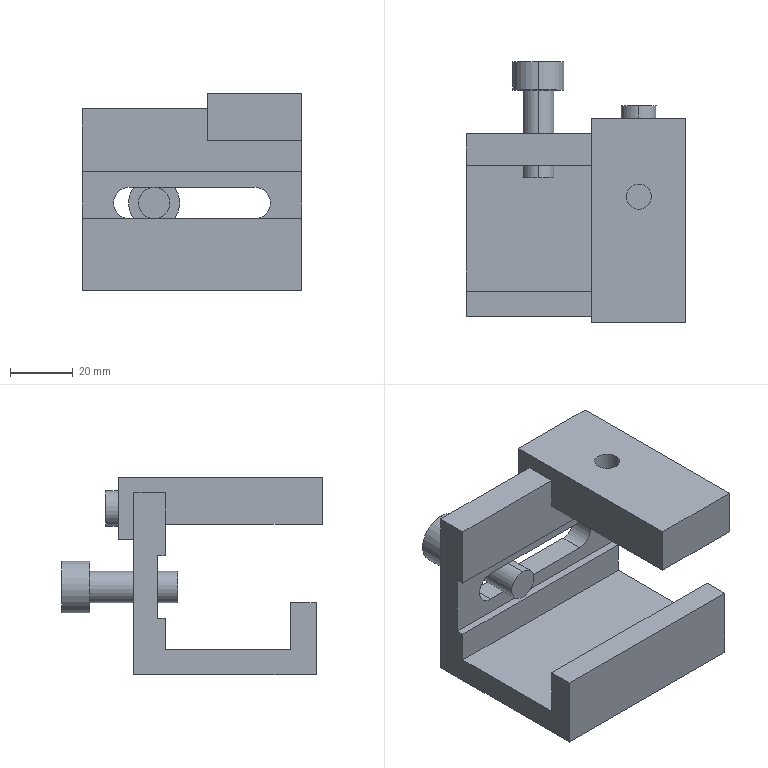Part | SolidWorks | features ICE 11, Extrusion 1 | 2 solids | 50 faces | box 70 x 83 x 63 mm | volume 98989 mm3 | plane 40 | cylinder 10 | commonest cylinder face diameters 10 x4 8 x2 11.171 x2 16.318 x2
STEP:
#1=CARTESIAN_POINT('',(22.948,33.,28.159));
#2=VERTEX_POINT('',#1);
#3=CARTESIAN_POINT('',(22.948,33.,11.841));
#4=VERTEX_POINT('',#3);
#5=CARTESIAN_POINT('',(22.948,33.,20.));
#6=DIRECTION('',(0.,1.,0.));
#7=DIRECTION('',(0.,0.,1.));
#8=AXIS2_PLACEMENT_3D('',#5,#6,#7);
#9=CIRCLE('',#8,8.159);
#10=EDGE_CURVE('',#2,#4,#9,.T.);
#11=ORIENTED_EDGE('',*,*,#10,.F.);
#12=CARTESIAN_POINT('',(22.948,24.,28.159));
#13=VERTEX_POINT('',#12);
#14=CARTESIAN_POINT('',(22.948,33.,28.159));
#15=DIRECTION('',(0.,-1.,0.));
#16=VECTOR('',#15,1000.);
#17=LINE('',#14,#16);
#18=EDGE_CURVE('',#2,#13,#17,.T.);
#19=ORIENTED_EDGE('',*,*,#18,.T.);
#20=CARTESIAN_POINT('',(22.948,24.,11.841));
#21=VERTEX_POINT('',#20);
#22=CARTESIAN_POINT('',(22.948,24.,20.));
#23=DIRECTION('',(0.,1.,0.));
#24=DIRECTION('',(0.,0.,1.));
#25=AXIS2_PLACEMENT_3D('',#22,#23,#24);
#26=CIRCLE('',#25,8.159);
#27=EDGE_CURVE('',#13,#21,#26,.T.);
#28=ORIENTED_EDGE('',*,*,#27,.T.);
#29=CARTESIAN_POINT('',(22.948,33.,11.841));
#30=DIRECTION('',(0.,-1.,0.));
#31=VECTOR('',#30,1000.);
#32=LINE('',#29,#31);
#33=EDGE_CURVE('',#4,#21,#32,.T.);
#34=ORIENTED_EDGE('',*,*,#33,.F.);
#35=EDGE_LOOP('',(#11,#19,#28,#34));
#36=FACE_OUTER_BOUND('',#35,.T.);
#37=CARTESIAN_POINT('',(22.948,33.,20.));
#38=DIRECTION('',(0.,-1.,0.));
#39=DIRECTION('',(0.,0.,-1.));
#40=AXIS2_PLACEMENT_3D('',#37,#38,#39);
#41=CYLINDRICAL_SURFACE('',#40,8.159);
#42=ADVANCED_FACE('',(#36),#41,.T.);
#43=CARTESIAN_POINT('',(22.948,24.,15.));
#44=VERTEX_POINT('',#43);
#45=CARTESIAN_POINT('',(22.948,24.,25.));
#46=VERTEX_POINT('',#45);
#47=CARTESIAN_POINT('',(22.948,24.,20.));
#48=DIRECTION('',(0.,-1.,0.));
#49=DIRECTION('',(0.,0.,-1.));
#50=AXIS2_PLACEMENT_3D('',#47,#48,#49);
#51=CIRCLE('',#50,5.);
#52=EDGE_CURVE('',#44,#46,#51,.T.);
#53=ORIENTED_EDGE('',*,*,#52,.T.);
#54=CARTESIAN_POINT('',(22.948,-4.,25.));
#55=VERTEX_POINT('',#54);
#56=CARTESIAN_POINT('',(22.948,24.,25.));
#57=DIRECTION('',(0.,-1.,0.));
#58=VECTOR('',#57,1000.);
#59=LINE('',#56,#58);
#60=EDGE_CURVE('',#46,#55,#59,.T.);
#61=ORIENTED_EDGE('',*,*,#60,.T.);
#62=CARTESIAN_POINT('',(22.948,-4.,15.));
#63=VERTEX_POINT('',#62);
#64=CARTESIAN_POINT('',(22.948,-4.,20.));
#65=DIRECTION('',(0.,-1.,0.));
#66=DIRECTION('',(0.,0.,-1.));
#67=AXIS2_PLACEMENT_3D('',#64,#65,#66);
#68=CIRCLE('',#67,5.);
#69=EDGE_CURVE('',#63,#55,#68,.T.);
#70=ORIENTED_EDGE('',*,*,#69,.F.);
#71=CARTESIAN_POINT('',(22.948,24.,15.));
#72=DIRECTION('',(0.,-1.,0.));
#73=VECTOR('',#72,1000.);
#74=LINE('',#71,#73);
#75=EDGE_CURVE('',#44,#63,#74,.T.);
#76=ORIENTED_EDGE('',*,*,#75,.F.);
#77=EDGE_LOOP('',(#53,#61,#70,#76));
#78=FACE_OUTER_BOUND('',#77,.T.);
#79=CARTESIAN_POINT('',(22.948,24.,20.));
#80=DIRECTION('',(0.,-1.,0.));
#81=DIRECTION('',(0.,0.,-1.));
#82=AXIS2_PLACEMENT_3D('',#79,#80,#81);
#83=CYLINDRICAL_SURFACE('',#82,5.);
#84=ADVANCED_FACE('',(#78),#83,.T.);
#85=ORIENTED_EDGE('',*,*,#60,.F.);
#86=CARTESIAN_POINT('',(22.948,24.,20.));
#87=DIRECTION('',(0.,-1.,0.));
#88=DIRECTION('',(0.,0.,-1.));
#89=AXIS2_PLACEMENT_3D('',#86,#87,#88);
#90=CIRCLE('',#89,5.);
#91=EDGE_CURVE('',#46,#44,#90,.T.);
#92=ORIENTED_EDGE('',*,*,#91,.T.);
#93=ORIENTED_EDGE('',*,*,#75,.T.);
#94=CARTESIAN_POINT('',(22.948,-4.,20.));
#95=DIRECTION('',(0.,-1.,0.));
#96=DIRECTION('',(0.,0.,-1.));
#97=AXIS2_PLACEMENT_3D('',#94,#95,#96);
#98=CIRCLE('',#97,5.);
#99=EDGE_CURVE('',#55,#63,#98,.T.);
#100=ORIENTED_EDGE('',*,*,#99,.F.);
#101=EDGE_LOOP('',(#85,#92,#93,#100));
#102=FACE_OUTER_BOUND('',#101,.T.);
#103=CARTESIAN_POINT('',(22.948,24.,20.));
#104=DIRECTION('',(0.,-1.,0.));
#105=DIRECTION('',(0.,0.,-1.));
#106=AXIS2_PLACEMENT_3D('',#103,#104,#105);
#107=CYLINDRICAL_SURFACE('',#106,5.);
#108=ADVANCED_FACE('',(#102),#107,.T.);
#109=ORIENTED_EDGE('',*,*,#69,.T.);
#110=ORIENTED_EDGE('',*,*,#99,.T.);
#111=EDGE_LOOP('',(#109,#110));
#112=FACE_OUTER_BOUND('',#111,.T.);
#113=CARTESIAN_POINT('',(22.948,-4.,20.));
#114=DIRECTION('',(0.,-1.,0.));
#115=DIRECTION('',(0.,0.,-1.));
#116=AXIS2_PLACEMENT_3D('',#113,#114,#115);
#117=PLANE('',#116);
#118=ADVANCED_FACE('',(#112),#117,.T.);
#119=ORIENTED_EDGE('',*,*,#18,.F.);
#120=CARTESIAN_POINT('',(22.948,33.,20.));
#121=DIRECTION('',(0.,1.,0.));
#122=DIRECTION('',(0.,0.,1.));
#123=AXIS2_PLACEMENT_3D('',#120,#121,#122);
#124=CIRCLE('',#123,8.159);
#125=EDGE_CURVE('',#4,#2,#124,.T.);
#126=ORIENTED_EDGE('',*,*,#125,.F.);
#127=ORIENTED_EDGE('',*,*,#33,.T.);
#128=CARTESIAN_POINT('',(22.948,24.,20.));
#129=DIRECTION('',(0.,1.,0.));
#130=DIRECTION('',(0.,0.,1.));
#131=AXIS2_PLACEMENT_3D('',#128,#129,#130);
#132=CIRCLE('',#131,8.159);
#133=EDGE_CURVE('',#21,#13,#132,.T.);
#134=ORIENTED_EDGE('',*,*,#133,.T.);
#135=EDGE_LOOP('',(#119,#126,#127,#134));
#136=FACE_OUTER_BOUND('',#135,.T.);
#137=CARTESIAN_POINT('',(22.948,33.,20.));
#138=DIRECTION('',(0.,-1.,0.));
#139=DIRECTION('',(0.,0.,-1.));
#140=AXIS2_PLACEMENT_3D('',#137,#138,#139);
#141=CYLINDRICAL_SURFACE('',#140,8.159);
#142=ADVANCED_FACE('',(#136),#141,.T.);
#143=CARTESIAN_POINT('',(23.272,33.,24.704));
#144=VERTEX_POINT('',#143);
#145=CARTESIAN_POINT('',(27.183,33.,22.071));
#146=VERTEX_POINT('',#145);
#147=CARTESIAN_POINT('',(23.272,33.,24.704));
#148=DIRECTION('',(0.8296,0.,-0.5584));
#149=VECTOR('',#148,1000.);
#150=LINE('',#147,#149);
#151=EDGE_CURVE('',#144,#146,#150,.T.);
#152=ORIENTED_EDGE('',*,*,#151,.F.);
#153=CARTESIAN_POINT('',(19.037,33.,22.633));
#154=VERTEX_POINT('',#153);
#155=CARTESIAN_POINT('',(19.037,33.,22.633));
#156=DIRECTION('',(0.8984,0.,0.4392));
#157=VECTOR('',#156,1000.);
#158=LINE('',#155,#157);
#159=EDGE_CURVE('',#154,#144,#158,.T.);
#160=ORIENTED_EDGE('',*,*,#159,.F.);
#161=CARTESIAN_POINT('',(18.712,33.,17.929));
#162=VERTEX_POINT('',#161);
#163=CARTESIAN_POINT('',(18.712,33.,17.929));
#164=DIRECTION('',(0.06882,0.,0.9976));
#165=VECTOR('',#164,1000.);
#166=LINE('',#163,#165);
#167=EDGE_CURVE('',#162,#154,#166,.T.);
#168=ORIENTED_EDGE('',*,*,#167,.F.);
#169=CARTESIAN_POINT('',(22.623,33.,15.296));
#170=VERTEX_POINT('',#169);
#171=CARTESIAN_POINT('',(22.623,33.,15.296));
#172=DIRECTION('',(-0.8296,0.,0.5584));
#173=VECTOR('',#172,1000.);
#174=LINE('',#171,#173);
#175=EDGE_CURVE('',#170,#162,#174,.T.);
#176=ORIENTED_EDGE('',*,*,#175,.F.);
#177=CARTESIAN_POINT('',(26.859,33.,17.367));
#178=VERTEX_POINT('',#177);
#179=CARTESIAN_POINT('',(26.859,33.,17.367));
#180=DIRECTION('',(-0.8984,0.,-0.4392));
#181=VECTOR('',#180,1000.);
#182=LINE('',#179,#181);
#183=EDGE_CURVE('',#178,#170,#182,.T.);
#184=ORIENTED_EDGE('',*,*,#183,.F.);
#185=CARTESIAN_POINT('',(27.183,33.,22.071));
#186=DIRECTION('',(-0.06882,0.,-0.9976));
#187=VECTOR('',#186,1000.);
#188=LINE('',#185,#187);
#189=EDGE_CURVE('',#146,#178,#188,.T.);
#190=ORIENTED_EDGE('',*,*,#189,.F.);
#191=EDGE_LOOP('',(#152,#160,#168,#176,#184,#190));
#192=FACE_BOUND('',#191,.T.);
#193=ORIENTED_EDGE('',*,*,#125,.T.);
#194=ORIENTED_EDGE('',*,*,#10,.T.);
#195=EDGE_LOOP('',(#193,#194));
#196=FACE_OUTER_BOUND('',#195,.T.);
#197=CARTESIAN_POINT('',(22.948,33.,20.));
#198=DIRECTION('',(0.,1.,0.));
#199=DIRECTION('',(0.,0.,1.));
#200=AXIS2_PLACEMENT_3D('',#197,#198,#199);
#201=PLANE('',#200);
#202=ADVANCED_FACE('',(#192,#196),#201,.T.);
#203=ORIENTED_EDGE('',*,*,#52,.F.);
#204=ORIENTED_EDGE('',*,*,#91,.F.);
#205=EDGE_LOOP('',(#203,#204));
#206=FACE_BOUND('',#205,.T.);
#207=ORIENTED_EDGE('',*,*,#133,.F.);
#208=ORIENTED_EDGE('',*,*,#27,.F.);
#209=EDGE_LOOP('',(#207,#208));
#210=FACE_OUTER_BOUND('',#209,.T.);
#211=CARTESIAN_POINT('',(22.948,24.,20.));
#212=DIRECTION('',(0.,1.,0.));
#213=DIRECTION('',(0.,0.,1.));
#214=AXIS2_PLACEMENT_3D('',#211,#212,#213);
#215=PLANE('',#214);
#216=ADVANCED_FACE('',(#206,#210),#215,.F.);
#217=ORIENTED_EDGE('',*,*,#151,.T.);
#218=CARTESIAN_POINT('',(27.183,26.,22.071));
#219=VERTEX_POINT('',#218);
#220=CARTESIAN_POINT('',(27.183,26.,22.071));
#221=DIRECTION('',(0.,1.,0.));
#222=VECTOR('',#221,1000.);
#223=LINE('',#220,#222);
#224=EDGE_CURVE('',#219,#146,#223,.T.);
#225=ORIENTED_EDGE('',*,*,#224,.F.);
#226=CARTESIAN_POINT('',(23.272,26.,24.704));
#227=VERTEX_POINT('',#226);
#228=CARTESIAN_POINT('',(23.272,26.,24.704));
#229=DIRECTION('',(0.8296,0.,-0.5584));
#230=VECTOR('',#229,1000.);
#231=LINE('',#228,#230);
#232=EDGE_CURVE('',#227,#219,#231,.T.);
#233=ORIENTED_EDGE('',*,*,#232,.F.);
#234=CARTESIAN_POINT('',(23.272,26.,24.704));
#235=DIRECTION('',(0.,1.,0.));
#236=VECTOR('',#235,1000.);
#237=LINE('',#234,#236);
#238=EDGE_CURVE('',#227,#144,#237,.T.);
#239=ORIENTED_EDGE('',*,*,#238,.T.);
#240=EDGE_LOOP('',(#217,#225,#233,#239));
#241=FACE_OUTER_BOUND('',#240,.T.);
#242=CARTESIAN_POINT('',(23.272,26.,24.704));
#243=DIRECTION('',(0.5584,0.,0.8296));
#244=DIRECTION('',(0.8296,0.,-0.5584));
#245=AXIS2_PLACEMENT_3D('',#242,#243,#244);
#246=PLANE('',#245);
#247=ADVANCED_FACE('',(#241),#246,.F.);
#248=ORIENTED_EDGE('',*,*,#159,.T.);
#249=ORIENTED_EDGE('',*,*,#238,.F.);
#250=CARTESIAN_POINT('',(19.037,26.,22.633));
#251=VERTEX_POINT('',#250);
#252=CARTESIAN_POINT('',(19.037,26.,22.633));
#253=DIRECTION('',(0.8984,0.,0.4392));
#254=VECTOR('',#253,1000.);
#255=LINE('',#252,#254);
#256=EDGE_CURVE('',#251,#227,#255,.T.);
#257=ORIENTED_EDGE('',*,*,#256,.F.);
#258=CARTESIAN_POINT('',(19.037,26.,22.633));
#259=DIRECTION('',(0.,1.,0.));
#260=VECTOR('',#259,1000.);
#261=LINE('',#258,#260);
#262=EDGE_CURVE('',#251,#154,#261,.T.);
#263=ORIENTED_EDGE('',*,*,#262,.T.);
#264=EDGE_LOOP('',(#248,#249,#257,#263));
#265=FACE_OUTER_BOUND('',#264,.T.);
#266=CARTESIAN_POINT('',(19.037,26.,22.633));
#267=DIRECTION('',(-0.4392,0.,0.8984));
#268=DIRECTION('',(0.8984,0.,0.4392));
#269=AXIS2_PLACEMENT_3D('',#266,#267,#268);
#270=PLANE('',#269);
#271=ADVANCED_FACE('',(#265),#270,.F.);
#272=ORIENTED_EDGE('',*,*,#167,.T.);
#273=ORIENTED_EDGE('',*,*,#262,.F.);
#274=CARTESIAN_POINT('',(18.712,26.,17.929));
#275=VERTEX_POINT('',#274);
#276=CARTESIAN_POINT('',(18.712,26.,17.929));
#277=DIRECTION('',(0.06882,0.,0.9976));
#278=VECTOR('',#277,1000.);
#279=LINE('',#276,#278);
#280=EDGE_CURVE('',#275,#251,#279,.T.);
#281=ORIENTED_EDGE('',*,*,#280,.F.);
#282=CARTESIAN_POINT('',(18.712,26.,17.929));
#283=DIRECTION('',(0.,1.,0.));
#284=VECTOR('',#283,1000.);
#285=LINE('',#282,#284);
#286=EDGE_CURVE('',#275,#162,#285,.T.);
#287=ORIENTED_EDGE('',*,*,#286,.T.);
#288=EDGE_LOOP('',(#272,#273,#281,#287));
#289=FACE_OUTER_BOUND('',#288,.T.);
#290=CARTESIAN_POINT('',(18.712,26.,17.929));
#291=DIRECTION('',(-0.9976,0.,0.06882));
#292=DIRECTION('',(0.06882,0.,0.9976));
#293=AXIS2_PLACEMENT_3D('',#290,#291,#292);
#294=PLANE('',#293);
#295=ADVANCED_FACE('',(#289),#294,.F.);
#296=ORIENTED_EDGE('',*,*,#175,.T.);
#297=ORIENTED_EDGE('',*,*,#286,.F.);
#298=CARTESIAN_POINT('',(22.623,26.,15.296));
#299=VERTEX_POINT('',#298);
#300=CARTESIAN_POINT('',(22.623,26.,15.296));
#301=DIRECTION('',(-0.8296,0.,0.5584));
#302=VECTOR('',#301,1000.);
#303=LINE('',#300,#302);
#304=EDGE_CURVE('',#299,#275,#303,.T.);
#305=ORIENTED_EDGE('',*,*,#304,.F.);
#306=CARTESIAN_POINT('',(22.623,26.,15.296));
#307=DIRECTION('',(0.,1.,0.));
#308=VECTOR('',#307,1000.);
#309=LINE('',#306,#308);
#310=EDGE_CURVE('',#299,#170,#309,.T.);
#311=ORIENTED_EDGE('',*,*,#310,.T.);
#312=EDGE_LOOP('',(#296,#297,#305,#311));
#313=FACE_OUTER_BOUND('',#312,.T.);
#314=CARTESIAN_POINT('',(22.623,26.,15.296));
#315=DIRECTION('',(-0.5584,0.,-0.8296));
#316=DIRECTION('',(-0.8296,0.,0.5584));
#317=AXIS2_PLACEMENT_3D('',#314,#315,#316);
#318=PLANE('',#317);
#319=ADVANCED_FACE('',(#313),#318,.F.);
#320=ORIENTED_EDGE('',*,*,#183,.T.);
#321=ORIENTED_EDGE('',*,*,#310,.F.);
#322=CARTESIAN_POINT('',(26.859,26.,17.367));
#323=VERTEX_POINT('',#322);
#324=CARTESIAN_POINT('',(26.859,26.,17.367));
#325=DIRECTION('',(-0.8984,0.,-0.4392));
#326=VECTOR('',#325,1000.);
#327=LINE('',#324,#326);
#328=EDGE_CURVE('',#323,#299,#327,.T.);
#329=ORIENTED_EDGE('',*,*,#328,.F.);
#330=CARTESIAN_POINT('',(26.859,26.,17.367));
#331=DIRECTION('',(0.,1.,0.));
#332=VECTOR('',#331,1000.);
#333=LINE('',#330,#332);
#334=EDGE_CURVE('',#323,#178,#333,.T.);
#335=ORIENTED_EDGE('',*,*,#334,.T.);
#336=EDGE_LOOP('',(#320,#321,#329,#335));
#337=FACE_OUTER_BOUND('',#336,.T.);
#338=CARTESIAN_POINT('',(26.859,26.,17.367));
#339=DIRECTION('',(0.4392,0.,-0.8984));
#340=DIRECTION('',(-0.8984,0.,-0.4392));
#341=AXIS2_PLACEMENT_3D('',#338,#339,#340);
#342=PLANE('',#341);
#343=ADVANCED_FACE('',(#337),#342,.F.);
#344=ORIENTED_EDGE('',*,*,#189,.T.);
#345=ORIENTED_EDGE('',*,*,#334,.F.);
#346=CARTESIAN_POINT('',(27.183,26.,22.071));
#347=DIRECTION('',(-0.06882,0.,-0.9976));
#348=VECTOR('',#347,1000.);
#349=LINE('',#346,#348);
#350=EDGE_CURVE('',#219,#323,#349,.T.);
#351=ORIENTED_EDGE('',*,*,#350,.F.);
#352=ORIENTED_EDGE('',*,*,#224,.T.);
#353=EDGE_LOOP('',(#344,#345,#351,#352));
#354=FACE_OUTER_BOUND('',#353,.T.);
#355=CARTESIAN_POINT('',(27.183,26.,22.071));
#356=DIRECTION('',(0.9976,0.,-0.06882));
#357=DIRECTION('',(-0.06882,0.,-0.9976));
#358=AXIS2_PLACEMENT_3D('',#355,#356,#357);
#359=PLANE('',#358);
#360=ADVANCED_FACE('',(#354),#359,.F.);
#361=ORIENTED_EDGE('',*,*,#232,.T.);
#362=ORIENTED_EDGE('',*,*,#350,.T.);
#363=ORIENTED_EDGE('',*,*,#328,.T.);
#364=ORIENTED_EDGE('',*,*,#304,.T.);
#365=ORIENTED_EDGE('',*,*,#280,.T.);
#366=ORIENTED_EDGE('',*,*,#256,.T.);
#367=EDGE_LOOP('',(#361,#362,#363,#364,#365,#366));
#368=FACE_OUTER_BOUND('',#367,.T.);
#369=CARTESIAN_POINT('',(0.,26.,0.));
#370=DIRECTION('',(0.,1.,0.));
#371=DIRECTION('',(0.,0.,1.));
#372=AXIS2_PLACEMENT_3D('',#369,#370,#371);
#373=PLANE('',#372);
#374=ADVANCED_FACE('',(#368),#373,.T.);
#375=CLOSED_SHELL('',(#42,#84,#108,#118,#142,#202,#216,#247,#271,#295,#319,#343,#360,#374));
#376=MANIFOLD_SOLID_BREP('',#375);
#377=CARTESIAN_POINT('',(59.,-10.,40.));
#378=VERTEX_POINT('',#377);
#379=CARTESIAN_POINT('',(51.,-10.,40.));
#380=VERTEX_POINT('',#379);
#381=CARTESIAN_POINT('',(55.,-10.,40.));
#382=DIRECTION('',(0.,0.,-1.));
#383=DIRECTION('',(1.,0.,0.));
#384=AXIS2_PLACEMENT_3D('',#381,#382,#383);
#385=CIRCLE('',#384,4.);
#386=EDGE_CURVE('',#378,#380,#385,.T.);
#387=ORIENTED_EDGE('',*,*,#386,.T.);
#388=CARTESIAN_POINT('',(51.,-10.,55.));
#389=VERTEX_POINT('',#388);
#390=CARTESIAN_POINT('',(51.,-10.,-0.001));
#391=DIRECTION('',(0.,0.,1.));
#392=VECTOR('',#391,1000.);
#393=LINE('',#390,#392);
#394=EDGE_CURVE('',#380,#389,#393,.T.);
#395=ORIENTED_EDGE('',*,*,#394,.T.);
#396=CARTESIAN_POINT('',(59.,-10.,55.));
#397=VERTEX_POINT('',#396);
#398=CARTESIAN_POINT('',(55.,-10.,55.));
#399=DIRECTION('',(0.,0.,1.));
#400=DIRECTION('',(1.,0.,0.));
#401=AXIS2_PLACEMENT_3D('',#398,#399,#400);
#402=CIRCLE('',#401,4.);
#403=EDGE_CURVE('',#389,#397,#402,.T.);
#404=ORIENTED_EDGE('',*,*,#403,.T.);
#405=CARTESIAN_POINT('',(59.,-10.,-0.001));
#406=DIRECTION('',(0.,0.,1.));
#407=VECTOR('',#406,1000.);
#408=LINE('',#405,#407);
#409=EDGE_CURVE('',#378,#397,#408,.T.);
#410=ORIENTED_EDGE('',*,*,#409,.F.);
#411=EDGE_LOOP('',(#387,#395,#404,#410));
#412=FACE_OUTER_BOUND('',#411,.T.);
#413=CARTESIAN_POINT('',(55.,-10.,-0.001));
#414=DIRECTION('',(0.,0.,1.));
#415=DIRECTION('',(1.,0.,0.));
#416=AXIS2_PLACEMENT_3D('',#413,#414,#415);
#417=CYLINDRICAL_SURFACE('',#416,4.);
#418=ADVANCED_FACE('',(#412),#417,.F.);
#419=CARTESIAN_POINT('',(55.,19.,50.585));
#420=VERTEX_POINT('',#419);
#421=CARTESIAN_POINT('',(55.,19.,39.415));
#422=VERTEX_POINT('',#421);
#423=CARTESIAN_POINT('',(55.,19.,45.));
#424=DIRECTION('',(0.,1.,0.));
#425=DIRECTION('',(0.,0.,1.));
#426=AXIS2_PLACEMENT_3D('',#423,#424,#425);
#427=CIRCLE('',#426,5.585);
#428=EDGE_CURVE('',#420,#422,#427,.T.);
#429=ORIENTED_EDGE('',*,*,#428,.F.);
#430=CARTESIAN_POINT('',(55.,15.,50.585));
#431=VERTEX_POINT('',#430);
#432=CARTESIAN_POINT('',(55.,19.,50.585));
#433=DIRECTION('',(0.,-1.,0.));
#434=VECTOR('',#433,1000.);
#435=LINE('',#432,#434);
#436=EDGE_CURVE('',#420,#431,#435,.T.);
#437=ORIENTED_EDGE('',*,*,#436,.T.);
#438=CARTESIAN_POINT('',(55.,15.,39.415));
#439=VERTEX_POINT('',#438);
#440=CARTESIAN_POINT('',(55.,15.,45.));
#441=DIRECTION('',(0.,1.,0.));
#442=DIRECTION('',(0.,0.,1.));
#443=AXIS2_PLACEMENT_3D('',#440,#441,#442);
#444=CIRCLE('',#443,5.585);
#445=EDGE_CURVE('',#431,#439,#444,.T.);
#446=ORIENTED_EDGE('',*,*,#445,.T.);
#447=CARTESIAN_POINT('',(55.,19.,39.415));
#448=DIRECTION('',(0.,-1.,0.));
#449=VECTOR('',#448,1000.);
#450=LINE('',#447,#449);
#451=EDGE_CURVE('',#422,#439,#450,.T.);
#452=ORIENTED_EDGE('',*,*,#451,.F.);
#453=EDGE_LOOP('',(#429,#437,#446,#452));
#454=FACE_OUTER_BOUND('',#453,.T.);
#455=CARTESIAN_POINT('',(55.,19.,45.));
#456=DIRECTION('',(0.,-1.,0.));
#457=DIRECTION('',(0.,0.,-1.));
#458=AXIS2_PLACEMENT_3D('',#455,#456,#457);
#459=CYLINDRICAL_SURFACE('',#458,5.585);
#460=ADVANCED_FACE('',(#454),#459,.T.);
#461=CARTESIAN_POINT('',(70.,15.,55.));
#462=VERTEX_POINT('',#461);
#463=CARTESIAN_POINT('',(70.,15.,35.));
#464=VERTEX_POINT('',#463);
#465=CARTESIAN_POINT('',(70.,15.,50.));
#466=DIRECTION('',(0.,0.,-1.));
#467=VECTOR('',#466,1000.);
#468=LINE('',#465,#467);
#469=EDGE_CURVE('',#462,#464,#468,.T.);
#470=ORIENTED_EDGE('',*,*,#469,.T.);
#471=CARTESIAN_POINT('',(40.,15.,35.));
#472=VERTEX_POINT('',#471);
#473=CARTESIAN_POINT('',(70.,15.,35.));
#474=DIRECTION('',(-1.,0.,0.));
#475=VECTOR('',#474,1000.);
#476=LINE('',#473,#475);
#477=EDGE_CURVE('',#464,#472,#476,.T.);
#478=ORIENTED_EDGE('',*,*,#477,.T.);
#479=CARTESIAN_POINT('',(40.,15.,55.));
#480=VERTEX_POINT('',#479);
#481=CARTESIAN_POINT('',(40.,15.,50.));
#482=DIRECTION('',(0.,0.,1.));
#483=VECTOR('',#482,1000.);
#484=LINE('',#481,#483);
#485=EDGE_CURVE('',#472,#480,#484,.T.);
#486=ORIENTED_EDGE('',*,*,#485,.T.);
#487=CARTESIAN_POINT('',(40.,15.,55.));
#488=DIRECTION('',(-1.,0.,0.));
#489=VECTOR('',#488,1000.);
#490=LINE('',#487,#489);
#491=EDGE_CURVE('',#462,#480,#490,.T.);
#492=ORIENTED_EDGE('',*,*,#491,.F.);
#493=EDGE_LOOP('',(#470,#478,#486,#492));
#494=FACE_OUTER_BOUND('',#493,.T.);
#495=CARTESIAN_POINT('',(55.,15.,45.));
#496=DIRECTION('',(0.,1.,0.));
#497=DIRECTION('',(0.,0.,1.));
#498=AXIS2_PLACEMENT_3D('',#495,#496,#497);
#499=CIRCLE('',#498,5.585);
#500=EDGE_CURVE('',#439,#431,#499,.T.);
#501=ORIENTED_EDGE('',*,*,#500,.F.);
#502=ORIENTED_EDGE('',*,*,#445,.F.);
#503=EDGE_LOOP('',(#501,#502));
#504=FACE_BOUND('',#503,.T.);
#505=CARTESIAN_POINT('',(0.,15.,0.));
#506=DIRECTION('',(0.,1.,0.));
#507=DIRECTION('',(0.,0.,1.));
#508=AXIS2_PLACEMENT_3D('',#505,#506,#507);
#509=PLANE('',#508);
#510=ADVANCED_FACE('',(#494,#504),#509,.T.);
#511=CARTESIAN_POINT('',(0.,0.,30.));
#512=VERTEX_POINT('',#511);
#513=CARTESIAN_POINT('',(0.,0.,50.));
#514=VERTEX_POINT('',#513);
#515=CARTESIAN_POINT('',(0.,0.,0.));
#516=DIRECTION('',(0.,0.,1.));
#517=VECTOR('',#516,1000.);
#518=LINE('',#515,#517);
#519=EDGE_CURVE('',#512,#514,#518,.T.);
#520=ORIENTED_EDGE('',*,*,#519,.F.);
#521=CARTESIAN_POINT('',(70.,0.,30.));
#522=VERTEX_POINT('',#521);
#523=CARTESIAN_POINT('',(70.001,0.,30.));
#524=DIRECTION('',(-1.,0.,0.));
#525=VECTOR('',#524,1000.);
#526=LINE('',#523,#525);
#527=EDGE_CURVE('',#522,#512,#526,.T.);
#528=ORIENTED_EDGE('',*,*,#527,.F.);
#529=CARTESIAN_POINT('',(70.,0.,40.));
#530=VERTEX_POINT('',#529);
#531=CARTESIAN_POINT('',(70.,0.,0.));
#532=DIRECTION('',(0.,0.,-1.));
#533=VECTOR('',#532,1000.);
#534=LINE('',#531,#533);
#535=EDGE_CURVE('',#530,#522,#534,.T.);
#536=ORIENTED_EDGE('',*,*,#535,.F.);
#537=CARTESIAN_POINT('',(40.,0.,40.));
#538=VERTEX_POINT('',#537);
#539=CARTESIAN_POINT('',(70.,0.,40.));
#540=DIRECTION('',(1.,0.,0.));
#541=VECTOR('',#540,1000.);
#542=LINE('',#539,#541);
#543=EDGE_CURVE('',#538,#530,#542,.T.);
#544=ORIENTED_EDGE('',*,*,#543,.F.);
#545=CARTESIAN_POINT('',(40.,0.,50.));
#546=VERTEX_POINT('',#545);
#547=CARTESIAN_POINT('',(40.,0.,50.));
#548=DIRECTION('',(0.,0.,-1.));
#549=VECTOR('',#548,1000.);
#550=LINE('',#547,#549);
#551=EDGE_CURVE('',#546,#538,#550,.T.);
#552=ORIENTED_EDGE('',*,*,#551,.F.);
#553=CARTESIAN_POINT('',(0.,0.,50.));
#554=DIRECTION('',(1.,0.,0.));
#555=VECTOR('',#554,1000.);
#556=LINE('',#553,#555);
#557=EDGE_CURVE('',#514,#546,#556,.T.);
#558=ORIENTED_EDGE('',*,*,#557,.F.);
#559=EDGE_LOOP('',(#520,#528,#536,#544,#552,#558));
#560=FACE_OUTER_BOUND('',#559,.T.);
#561=CARTESIAN_POINT('',(0.,0.,0.));
#562=DIRECTION('',(0.,1.,0.));
#563=DIRECTION('',(0.,0.,1.));
#564=AXIS2_PLACEMENT_3D('',#561,#562,#563);
#565=PLANE('',#564);
#566=ADVANCED_FACE('',(#560),#565,.F.);
#567=CARTESIAN_POINT('',(40.,10.,50.));
#568=VERTEX_POINT('',#567);
#569=CARTESIAN_POINT('',(40.,15.,50.));
#570=DIRECTION('',(0.,-1.,0.));
#571=VECTOR('',#570,1000.);
#572=LINE('',#569,#571);
#573=EDGE_CURVE('',#568,#546,#572,.T.);
#574=ORIENTED_EDGE('',*,*,#573,.F.);
#575=CARTESIAN_POINT('',(0.,10.,50.));
#576=VERTEX_POINT('',#575);
#577=CARTESIAN_POINT('',(0.,10.,50.));
#578=DIRECTION('',(1.,0.,0.));
#579=VECTOR('',#578,1000.);
#580=LINE('',#577,#579);
#581=EDGE_CURVE('',#576,#568,#580,.T.);
#582=ORIENTED_EDGE('',*,*,#581,.F.);
#583=CARTESIAN_POINT('',(0.,10.,50.));
#584=DIRECTION('',(0.,-1.,0.));
#585=VECTOR('',#584,1000.);
#586=LINE('',#583,#585);
#587=EDGE_CURVE('',#576,#514,#586,.T.);
#588=ORIENTED_EDGE('',*,*,#587,.T.);
#589=ORIENTED_EDGE('',*,*,#557,.T.);
#590=EDGE_LOOP('',(#574,#582,#588,#589));
#591=FACE_OUTER_BOUND('',#590,.T.);
#592=CARTESIAN_POINT('',(0.,10.,50.));
#593=DIRECTION('',(0.,0.,-1.));
#594=DIRECTION('',(-1.,0.,0.));
#595=AXIS2_PLACEMENT_3D('',#592,#593,#594);
#596=PLANE('',#595);
#597=ADVANCED_FACE('',(#591),#596,.F.);
#598=CARTESIAN_POINT('',(70.,0.,10.));
#599=VERTEX_POINT('',#598);
#600=CARTESIAN_POINT('',(70.,0.,0.));
#601=VERTEX_POINT('',#600);
#602=CARTESIAN_POINT('',(70.,0.,0.));
#603=DIRECTION('',(0.,0.,-1.));
#604=VECTOR('',#603,1000.);
#605=LINE('',#602,#604);
#606=EDGE_CURVE('',#599,#601,#605,.T.);
#607=ORIENTED_EDGE('',*,*,#606,.F.);
#608=CARTESIAN_POINT('',(0.,0.,10.));
#609=VERTEX_POINT('',#608);
#610=CARTESIAN_POINT('',(70.001,0.,10.));
#611=DIRECTION('',(1.,0.,0.));
#612=VECTOR('',#611,1000.);
#613=LINE('',#610,#612);
#614=EDGE_CURVE('',#609,#599,#613,.T.);
#615=ORIENTED_EDGE('',*,*,#614,.F.);
#616=CARTESIAN_POINT('',(0.,0.,0.));
#617=VERTEX_POINT('',#616);
#618=CARTESIAN_POINT('',(0.,0.,0.));
#619=DIRECTION('',(0.,0.,1.));
#620=VECTOR('',#619,1000.);
#621=LINE('',#618,#620);
#622=EDGE_CURVE('',#617,#609,#621,.T.);
#623=ORIENTED_EDGE('',*,*,#622,.F.);
#624=CARTESIAN_POINT('',(0.,0.,0.));
#625=DIRECTION('',(-1.,0.,0.));
#626=VECTOR('',#625,1000.);
#627=LINE('',#624,#626);
#628=EDGE_CURVE('',#601,#617,#627,.T.);
#629=ORIENTED_EDGE('',*,*,#628,.F.);
#630=EDGE_LOOP('',(#607,#615,#623,#629));
#631=FACE_OUTER_BOUND('',#630,.T.);
#632=CARTESIAN_POINT('',(0.,0.,0.));
#633=DIRECTION('',(0.,1.,0.));
#634=DIRECTION('',(0.,0.,1.));
#635=AXIS2_PLACEMENT_3D('',#632,#633,#634);
#636=PLANE('',#635);
#637=ADVANCED_FACE('',(#631),#636,.F.);
#638=CARTESIAN_POINT('',(0.,2.5,30.));
#639=VERTEX_POINT('',#638);
#640=CARTESIAN_POINT('',(0.,2.5,10.));
#641=VERTEX_POINT('',#640);
#642=CARTESIAN_POINT('',(0.,2.5,10.));
#643=DIRECTION('',(0.,0.,-1.));
#644=VECTOR('',#643,1000.);
#645=LINE('',#642,#644);
#646=EDGE_CURVE('',#639,#641,#645,.T.);
#647=ORIENTED_EDGE('',*,*,#646,.F.);
#648=CARTESIAN_POINT('',(0.,2.5,30.));
#649=DIRECTION('',(0.,1.,0.));
#650=VECTOR('',#649,1000.);
#651=LINE('',#648,#650);
#652=EDGE_CURVE('',#512,#639,#651,.T.);
#653=ORIENTED_EDGE('',*,*,#652,.F.);
#654=ORIENTED_EDGE('',*,*,#519,.T.);
#655=ORIENTED_EDGE('',*,*,#587,.F.);
#656=CARTESIAN_POINT('',(0.,10.,-8.));
#657=VERTEX_POINT('',#656);
#658=CARTESIAN_POINT('',(0.,10.,0.));
#659=DIRECTION('',(0.,0.,1.));
#660=VECTOR('',#659,1000.);
#661=LINE('',#658,#660);
#662=EDGE_CURVE('',#657,#576,#661,.T.);
#663=ORIENTED_EDGE('',*,*,#662,.F.);
#664=CARTESIAN_POINT('',(0.,-48.,-8.));
#665=VERTEX_POINT('',#664);
#666=CARTESIAN_POINT('',(0.,10.,-8.));
#667=DIRECTION('',(0.,-1.,0.));
#668=VECTOR('',#667,1000.);
#669=LINE('',#666,#668);
#670=EDGE_CURVE('',#657,#665,#669,.T.);
#671=ORIENTED_EDGE('',*,*,#670,.T.);
#672=CARTESIAN_POINT('',(0.,-48.,15.));
#673=VERTEX_POINT('',#672);
#674=CARTESIAN_POINT('',(0.,-48.,-8.));
#675=DIRECTION('',(0.,0.,1.));
#676=VECTOR('',#675,1000.);
#677=LINE('',#674,#676);
#678=EDGE_CURVE('',#665,#673,#677,.T.);
#679=ORIENTED_EDGE('',*,*,#678,.T.);
#680=CARTESIAN_POINT('',(0.,-40.,15.));
#681=VERTEX_POINT('',#680);
#682=CARTESIAN_POINT('',(0.,-48.,15.));
#683=DIRECTION('',(0.,1.,0.));
#684=VECTOR('',#683,1000.);
#685=LINE('',#682,#684);
#686=EDGE_CURVE('',#673,#681,#685,.T.);
#687=ORIENTED_EDGE('',*,*,#686,.T.);
#688=CARTESIAN_POINT('',(0.,-40.,0.));
#689=VERTEX_POINT('',#688);
#690=CARTESIAN_POINT('',(0.,-40.,15.));
#691=DIRECTION('',(0.,0.,-1.));
#692=VECTOR('',#691,1000.);
#693=LINE('',#690,#692);
#694=EDGE_CURVE('',#681,#689,#693,.T.);
#695=ORIENTED_EDGE('',*,*,#694,.T.);
#696=CARTESIAN_POINT('',(0.,-40.,0.));
#697=DIRECTION('',(0.,1.,0.));
#698=VECTOR('',#697,1000.);
#699=LINE('',#696,#698);
#700=EDGE_CURVE('',#689,#617,#699,.T.);
#701=ORIENTED_EDGE('',*,*,#700,.T.);
#702=ORIENTED_EDGE('',*,*,#622,.T.);
#703=CARTESIAN_POINT('',(0.,2.5,10.));
#704=DIRECTION('',(0.,-1.,0.));
#705=VECTOR('',#704,1000.);
#706=LINE('',#703,#705);
#707=EDGE_CURVE('',#641,#609,#706,.T.);
#708=ORIENTED_EDGE('',*,*,#707,.F.);
#709=EDGE_LOOP('',(#647,#653,#654,#655,#663,#671,#679,#687,#695,#701,#702,#708));
#710=FACE_OUTER_BOUND('',#709,.T.);
#711=CARTESIAN_POINT('',(0.,10.,0.));
#712=DIRECTION('',(1.,0.,0.));
#713=DIRECTION('',(0.,0.,-1.));
#714=AXIS2_PLACEMENT_3D('',#711,#712,#713);
#715=PLANE('',#714);
#716=ADVANCED_FACE('',(#710),#715,.F.);
#717=ORIENTED_EDGE('',*,*,#535,.T.);
#718=CARTESIAN_POINT('',(70.,2.5,30.));
#719=VERTEX_POINT('',#718);
#720=CARTESIAN_POINT('',(70.,2.5,30.));
#721=DIRECTION('',(0.,-1.,0.));
#722=VECTOR('',#721,1000.);
#723=LINE('',#720,#722);
#724=EDGE_CURVE('',#719,#522,#723,.T.);
#725=ORIENTED_EDGE('',*,*,#724,.F.);
#726=CARTESIAN_POINT('',(70.,2.5,10.));
#727=VERTEX_POINT('',#726);
#728=CARTESIAN_POINT('',(70.,2.5,10.));
#729=DIRECTION('',(0.,0.,1.));
#730=VECTOR('',#729,1000.);
#731=LINE('',#728,#730);
#732=EDGE_CURVE('',#727,#719,#731,.T.);
#733=ORIENTED_EDGE('',*,*,#732,.F.);
#734=CARTESIAN_POINT('',(70.,2.5,10.));
#735=DIRECTION('',(0.,1.,0.));
#736=VECTOR('',#735,1000.);
#737=LINE('',#734,#736);
#738=EDGE_CURVE('',#599,#727,#737,.T.);
#739=ORIENTED_EDGE('',*,*,#738,.F.);
#740=ORIENTED_EDGE('',*,*,#606,.T.);
#741=CARTESIAN_POINT('',(70.,-40.,0.));
#742=VERTEX_POINT('',#741);
#743=CARTESIAN_POINT('',(70.,-40.,0.));
#744=DIRECTION('',(0.,-1.,0.));
#745=VECTOR('',#744,1000.);
#746=LINE('',#743,#745);
#747=EDGE_CURVE('',#601,#742,#746,.T.);
#748=ORIENTED_EDGE('',*,*,#747,.T.);
#749=CARTESIAN_POINT('',(70.,-40.,15.));
#750=VERTEX_POINT('',#749);
#751=CARTESIAN_POINT('',(70.,-40.,15.));
#752=DIRECTION('',(0.,0.,1.));
#753=VECTOR('',#752,1000.);
#754=LINE('',#751,#753);
#755=EDGE_CURVE('',#742,#750,#754,.T.);
#756=ORIENTED_EDGE('',*,*,#755,.T.);
#757=CARTESIAN_POINT('',(70.,-48.,15.));
#758=VERTEX_POINT('',#757);
#759=CARTESIAN_POINT('',(70.,-48.,15.));
#760=DIRECTION('',(0.,-1.,0.));
#761=VECTOR('',#760,1000.);
#762=LINE('',#759,#761);
#763=EDGE_CURVE('',#750,#758,#762,.T.);
#764=ORIENTED_EDGE('',*,*,#763,.T.);
#765=CARTESIAN_POINT('',(70.,-48.,-8.));
#766=VERTEX_POINT('',#765);
#767=CARTESIAN_POINT('',(70.,-48.,-8.));
#768=DIRECTION('',(0.,0.,-1.));
#769=VECTOR('',#768,1000.);
#770=LINE('',#767,#769);
#771=EDGE_CURVE('',#758,#766,#770,.T.);
#772=ORIENTED_EDGE('',*,*,#771,.T.);
#773=CARTESIAN_POINT('',(70.,10.,-8.));
#774=VERTEX_POINT('',#773);
#775=CARTESIAN_POINT('',(70.,10.,-8.));
#776=DIRECTION('',(0.,1.,0.));
#777=VECTOR('',#776,1000.);
#778=LINE('',#775,#777);
#779=EDGE_CURVE('',#766,#774,#778,.T.);
#780=ORIENTED_EDGE('',*,*,#779,.T.);
#781=CARTESIAN_POINT('',(70.,10.,35.));
#782=VERTEX_POINT('',#781);
#783=CARTESIAN_POINT('',(70.,10.,0.));
#784=DIRECTION('',(0.,0.,-1.));
#785=VECTOR('',#784,1000.);
#786=LINE('',#783,#785);
#787=EDGE_CURVE('',#782,#774,#786,.T.);
#788=ORIENTED_EDGE('',*,*,#787,.F.);
#789=CARTESIAN_POINT('',(70.,15.,35.));
#790=DIRECTION('',(0.,-1.,0.));
#791=VECTOR('',#790,1000.);
#792=LINE('',#789,#791);
#793=EDGE_CURVE('',#464,#782,#792,.T.);
#794=ORIENTED_EDGE('',*,*,#793,.F.);
#795=ORIENTED_EDGE('',*,*,#469,.F.);
#796=CARTESIAN_POINT('',(70.,-50.,55.));
#797=VERTEX_POINT('',#796);
#798=CARTESIAN_POINT('',(70.,15.,55.));
#799=DIRECTION('',(0.,1.,0.));
#800=VECTOR('',#799,1000.);
#801=LINE('',#798,#800);
#802=EDGE_CURVE('',#797,#462,#801,.T.);
#803=ORIENTED_EDGE('',*,*,#802,.F.);
#804=CARTESIAN_POINT('',(70.,-50.,40.));
#805=VERTEX_POINT('',#804);
#806=CARTESIAN_POINT('',(70.,-50.,50.));
#807=DIRECTION('',(0.,0.,1.));
#808=VECTOR('',#807,1000.);
#809=LINE('',#806,#808);
#810=EDGE_CURVE('',#805,#797,#809,.T.);
#811=ORIENTED_EDGE('',*,*,#810,.F.);
#812=CARTESIAN_POINT('',(70.,-50.,40.));
#813=DIRECTION('',(0.,1.,0.));
#814=VECTOR('',#813,1000.);
#815=LINE('',#812,#814);
#816=EDGE_CURVE('',#805,#530,#815,.T.);
#817=ORIENTED_EDGE('',*,*,#816,.T.);
#818=EDGE_LOOP('',(#717,#725,#733,#739,#740,#748,#756,#764,#772,#780,#788,#794,#795,#803,#811,#817));
#819=FACE_OUTER_BOUND('',#818,.T.);
#820=CARTESIAN_POINT('',(70.,10.,0.));
#821=DIRECTION('',(-1.,0.,0.));
#822=DIRECTION('',(0.,0.,1.));
#823=AXIS2_PLACEMENT_3D('',#820,#821,#822);
#824=PLANE('',#823);
#825=ADVANCED_FACE('',(#819),#824,.F.);
#826=CARTESIAN_POINT('',(15.,10.,15.));
#827=VERTEX_POINT('',#826);
#828=CARTESIAN_POINT('',(15.,10.,25.));
#829=VERTEX_POINT('',#828);
#830=CARTESIAN_POINT('',(15.,10.,20.));
#831=DIRECTION('',(0.,1.,0.));
#832=DIRECTION('',(0.,0.,1.));
#833=AXIS2_PLACEMENT_3D('',#830,#831,#832);
#834=CIRCLE('',#833,5.);
#835=EDGE_CURVE('',#827,#829,#834,.T.);
#836=ORIENTED_EDGE('',*,*,#835,.F.);
#837=CARTESIAN_POINT('',(55.,10.,15.));
#838=VERTEX_POINT('',#837);
#839=CARTESIAN_POINT('',(15.,10.,15.));
#840=DIRECTION('',(-1.,0.,0.));
#841=VECTOR('',#840,1000.);
#842=LINE('',#839,#841);
#843=EDGE_CURVE('',#838,#827,#842,.T.);
#844=ORIENTED_EDGE('',*,*,#843,.F.);
#845=CARTESIAN_POINT('',(55.,10.,25.));
#846=VERTEX_POINT('',#845);
#847=CARTESIAN_POINT('',(55.,10.,20.));
#848=DIRECTION('',(0.,1.,0.));
#849=DIRECTION('',(0.,0.,1.));
#850=AXIS2_PLACEMENT_3D('',#847,#848,#849);
#851=CIRCLE('',#850,5.);
#852=EDGE_CURVE('',#846,#838,#851,.T.);
#853=ORIENTED_EDGE('',*,*,#852,.F.);
#854=CARTESIAN_POINT('',(15.,10.,25.));
#855=DIRECTION('',(1.,0.,0.));
#856=VECTOR('',#855,1000.);
#857=LINE('',#854,#856);
#858=EDGE_CURVE('',#829,#846,#857,.T.);
#859=ORIENTED_EDGE('',*,*,#858,.F.);
#860=EDGE_LOOP('',(#836,#844,#853,#859));
#861=FACE_BOUND('',#860,.T.);
#862=CARTESIAN_POINT('',(40.,10.,35.));
#863=VERTEX_POINT('',#862);
#864=CARTESIAN_POINT('',(40.,10.,50.));
#865=DIRECTION('',(0.,0.,1.));
#866=VECTOR('',#865,1000.);
#867=LINE('',#864,#866);
#868=EDGE_CURVE('',#863,#568,#867,.T.);
#869=ORIENTED_EDGE('',*,*,#868,.F.);
#870=CARTESIAN_POINT('',(70.,10.,35.));
#871=DIRECTION('',(-1.,0.,0.));
#872=VECTOR('',#871,1000.);
#873=LINE('',#870,#872);
#874=EDGE_CURVE('',#782,#863,#873,.T.);
#875=ORIENTED_EDGE('',*,*,#874,.F.);
#876=ORIENTED_EDGE('',*,*,#787,.T.);
#877=CARTESIAN_POINT('',(132.394,10.,-8.));
#878=DIRECTION('',(-1.,0.,0.));
#879=VECTOR('',#878,1000.);
#880=LINE('',#877,#879);
#881=EDGE_CURVE('',#774,#657,#880,.T.);
#882=ORIENTED_EDGE('',*,*,#881,.T.);
#883=ORIENTED_EDGE('',*,*,#662,.T.);
#884=ORIENTED_EDGE('',*,*,#581,.T.);
#885=EDGE_LOOP('',(#869,#875,#876,#882,#883,#884));
#886=FACE_OUTER_BOUND('',#885,.T.);
#887=CARTESIAN_POINT('',(0.,10.,0.));
#888=DIRECTION('',(0.,1.,0.));
#889=DIRECTION('',(0.,0.,1.));
#890=AXIS2_PLACEMENT_3D('',#887,#888,#889);
#891=PLANE('',#890);
#892=ADVANCED_FACE('',(#861,#886),#891,.T.);
#893=ORIENTED_EDGE('',*,*,#551,.T.);
#894=CARTESIAN_POINT('',(40.,-50.,40.));
#895=VERTEX_POINT('',#894);
#896=CARTESIAN_POINT('',(40.,-50.,40.));
#897=DIRECTION('',(0.,1.,0.));
#898=VECTOR('',#897,1000.);
#899=LINE('',#896,#898);
#900=EDGE_CURVE('',#895,#538,#899,.T.);
#901=ORIENTED_EDGE('',*,*,#900,.F.);
#902=CARTESIAN_POINT('',(40.,-50.,55.));
#903=VERTEX_POINT('',#902);
#904=CARTESIAN_POINT('',(40.,-50.,50.));
#905=DIRECTION('',(0.,0.,-1.));
#906=VECTOR('',#905,1000.);
#907=LINE('',#904,#906);
#908=EDGE_CURVE('',#903,#895,#907,.T.);
#909=ORIENTED_EDGE('',*,*,#908,.F.);
#910=CARTESIAN_POINT('',(40.,15.,55.));
#911=DIRECTION('',(0.,-1.,0.));
#912=VECTOR('',#911,1000.);
#913=LINE('',#910,#912);
#914=EDGE_CURVE('',#480,#903,#913,.T.);
#915=ORIENTED_EDGE('',*,*,#914,.F.);
#916=ORIENTED_EDGE('',*,*,#485,.F.);
#917=CARTESIAN_POINT('',(40.,15.,35.));
#918=DIRECTION('',(0.,-1.,0.));
#919=VECTOR('',#918,1000.);
#920=LINE('',#917,#919);
#921=EDGE_CURVE('',#472,#863,#920,.T.);
#922=ORIENTED_EDGE('',*,*,#921,.T.);
#923=ORIENTED_EDGE('',*,*,#868,.T.);
#924=ORIENTED_EDGE('',*,*,#573,.T.);
#925=EDGE_LOOP('',(#893,#901,#909,#915,#916,#922,#923,#924));
#926=FACE_OUTER_BOUND('',#925,.T.);
#927=CARTESIAN_POINT('',(40.,-50.,50.));
#928=DIRECTION('',(1.,0.,0.));
#929=DIRECTION('',(0.,0.,-1.));
#930=AXIS2_PLACEMENT_3D('',#927,#928,#929);
#931=PLANE('',#930);
#932=ADVANCED_FACE('',(#926),#931,.F.);
#933=ORIENTED_EDGE('',*,*,#386,.F.);
#934=CARTESIAN_POINT('',(55.,-10.,40.));
#935=DIRECTION('',(0.,0.,-1.));
#936=DIRECTION('',(1.,0.,0.));
#937=AXIS2_PLACEMENT_3D('',#934,#935,#936);
#938=CIRCLE('',#937,4.);
#939=EDGE_CURVE('',#380,#378,#938,.T.);
#940=ORIENTED_EDGE('',*,*,#939,.F.);
#941=EDGE_LOOP('',(#933,#940));
#942=FACE_BOUND('',#941,.T.);
#943=ORIENTED_EDGE('',*,*,#543,.T.);
#944=ORIENTED_EDGE('',*,*,#816,.F.);
#945=CARTESIAN_POINT('',(70.,-50.,40.));
#946=DIRECTION('',(1.,0.,0.));
#947=VECTOR('',#946,1000.);
#948=LINE('',#945,#947);
#949=EDGE_CURVE('',#895,#805,#948,.T.);
#950=ORIENTED_EDGE('',*,*,#949,.F.);
#951=ORIENTED_EDGE('',*,*,#900,.T.);
#952=EDGE_LOOP('',(#943,#944,#950,#951));
#953=FACE_OUTER_BOUND('',#952,.T.);
#954=CARTESIAN_POINT('',(70.,-50.,40.));
#955=DIRECTION('',(0.,0.,1.));
#956=DIRECTION('',(1.,0.,0.));
#957=AXIS2_PLACEMENT_3D('',#954,#955,#956);
#958=PLANE('',#957);
#959=ADVANCED_FACE('',(#942,#953),#958,.F.);
#960=ORIENTED_EDGE('',*,*,#810,.T.);
#961=CARTESIAN_POINT('',(40.,-50.,55.));
#962=DIRECTION('',(1.,0.,0.));
#963=VECTOR('',#962,1000.);
#964=LINE('',#961,#963);
#965=EDGE_CURVE('',#903,#797,#964,.T.);
#966=ORIENTED_EDGE('',*,*,#965,.F.);
#967=ORIENTED_EDGE('',*,*,#908,.T.);
#968=ORIENTED_EDGE('',*,*,#949,.T.);
#969=EDGE_LOOP('',(#960,#966,#967,#968));
#970=FACE_OUTER_BOUND('',#969,.T.);
#971=CARTESIAN_POINT('',(0.,-50.,0.));
#972=DIRECTION('',(0.,1.,0.));
#973=DIRECTION('',(0.,0.,1.));
#974=AXIS2_PLACEMENT_3D('',#971,#972,#973);
#975=PLANE('',#974);
#976=ADVANCED_FACE('',(#970),#975,.F.);
#977=ORIENTED_EDGE('',*,*,#874,.T.);
#978=ORIENTED_EDGE('',*,*,#921,.F.);
#979=ORIENTED_EDGE('',*,*,#477,.F.);
#980=ORIENTED_EDGE('',*,*,#793,.T.);
#981=EDGE_LOOP('',(#977,#978,#979,#980));
#982=FACE_OUTER_BOUND('',#981,.T.);
#983=CARTESIAN_POINT('',(70.,15.,35.));
#984=DIRECTION('',(0.,0.,1.));
#985=DIRECTION('',(1.,0.,0.));
#986=AXIS2_PLACEMENT_3D('',#983,#984,#985);
#987=PLANE('',#986);
#988=ADVANCED_FACE('',(#982),#987,.F.);
#989=CARTESIAN_POINT('',(55.,-10.,55.));
#990=DIRECTION('',(0.,0.,1.));
#991=DIRECTION('',(1.,0.,0.));
#992=AXIS2_PLACEMENT_3D('',#989,#990,#991);
#993=CIRCLE('',#992,4.);
#994=EDGE_CURVE('',#397,#389,#993,.T.);
#995=ORIENTED_EDGE('',*,*,#994,.F.);
#996=ORIENTED_EDGE('',*,*,#403,.F.);
#997=EDGE_LOOP('',(#995,#996));
#998=FACE_BOUND('',#997,.T.);
#999=ORIENTED_EDGE('',*,*,#914,.T.);
#1000=ORIENTED_EDGE('',*,*,#965,.T.);
#1001=ORIENTED_EDGE('',*,*,#802,.T.);
#1002=ORIENTED_EDGE('',*,*,#491,.T.);
#1003=EDGE_LOOP('',(#999,#1000,#1001,#1002));
#1004=FACE_OUTER_BOUND('',#1003,.T.);
#1005=CARTESIAN_POINT('',(0.,0.,55.));
#1006=DIRECTION('',(0.,0.,1.));
#1007=DIRECTION('',(1.,0.,0.));
#1008=AXIS2_PLACEMENT_3D('',#1005,#1006,#1007);
#1009=PLANE('',#1008);
#1010=ADVANCED_FACE('',(#998,#1004),#1009,.T.);
#1011=CARTESIAN_POINT('',(15.,2.5,25.));
#1012=VERTEX_POINT('',#1011);
#1013=CARTESIAN_POINT('',(15.,0.,25.));
#1014=DIRECTION('',(0.,1.,0.));
#1015=VECTOR('',#1014,1000.);
#1016=LINE('',#1013,#1015);
#1017=EDGE_CURVE('',#1012,#829,#1016,.T.);
#1018=ORIENTED_EDGE('',*,*,#1017,.F.);
#1019=CARTESIAN_POINT('',(15.,2.5,15.));
#1020=VERTEX_POINT('',#1019);
#1021=CARTESIAN_POINT('',(15.,2.5,20.));
#1022=DIRECTION('',(0.,1.,0.));
#1023=DIRECTION('',(0.,0.,1.));
#1024=AXIS2_PLACEMENT_3D('',#1021,#1022,#1023);
#1025=CIRCLE('',#1024,5.);
#1026=EDGE_CURVE('',#1020,#1012,#1025,.T.);
#1027=ORIENTED_EDGE('',*,*,#1026,.F.);
#1028=CARTESIAN_POINT('',(15.,0.,15.));
#1029=DIRECTION('',(0.,1.,0.));
#1030=VECTOR('',#1029,1000.);
#1031=LINE('',#1028,#1030);
#1032=EDGE_CURVE('',#1020,#827,#1031,.T.);
#1033=ORIENTED_EDGE('',*,*,#1032,.T.);
#1034=ORIENTED_EDGE('',*,*,#835,.T.);
#1035=EDGE_LOOP('',(#1018,#1027,#1033,#1034));
#1036=FACE_OUTER_BOUND('',#1035,.T.);
#1037=CARTESIAN_POINT('',(15.,0.,20.));
#1038=DIRECTION('',(0.,1.,0.));
#1039=DIRECTION('',(0.,0.,1.));
#1040=AXIS2_PLACEMENT_3D('',#1037,#1038,#1039);
#1041=CYLINDRICAL_SURFACE('',#1040,5.);
#1042=ADVANCED_FACE('',(#1036),#1041,.F.);
#1043=ORIENTED_EDGE('',*,*,#843,.T.);
#1044=ORIENTED_EDGE('',*,*,#1032,.F.);
#1045=CARTESIAN_POINT('',(55.,2.5,15.));
#1046=VERTEX_POINT('',#1045);
#1047=CARTESIAN_POINT('',(70.001,2.5,15.));
#1048=DIRECTION('',(-1.,0.,0.));
#1049=VECTOR('',#1048,1000.);
#1050=LINE('',#1047,#1049);
#1051=EDGE_CURVE('',#1046,#1020,#1050,.T.);
#1052=ORIENTED_EDGE('',*,*,#1051,.F.);
#1053=CARTESIAN_POINT('',(55.,0.,15.));
#1054=DIRECTION('',(0.,1.,0.));
#1055=VECTOR('',#1054,1000.);
#1056=LINE('',#1053,#1055);
#1057=EDGE_CURVE('',#1046,#838,#1056,.T.);
#1058=ORIENTED_EDGE('',*,*,#1057,.T.);
#1059=EDGE_LOOP('',(#1043,#1044,#1052,#1058));
#1060=FACE_OUTER_BOUND('',#1059,.T.);
#1061=CARTESIAN_POINT('',(15.,0.,15.));
#1062=DIRECTION('',(0.,0.,-1.));
#1063=DIRECTION('',(-1.,0.,0.));
#1064=AXIS2_PLACEMENT_3D('',#1061,#1062,#1063);
#1065=PLANE('',#1064);
#1066=ADVANCED_FACE('',(#1060),#1065,.F.);
#1067=ORIENTED_EDGE('',*,*,#1057,.F.);
#1068=CARTESIAN_POINT('',(55.,2.5,25.));
#1069=VERTEX_POINT('',#1068);
#1070=CARTESIAN_POINT('',(55.,2.5,20.));
#1071=DIRECTION('',(0.,1.,0.));
#1072=DIRECTION('',(0.,0.,1.));
#1073=AXIS2_PLACEMENT_3D('',#1070,#1071,#1072);
#1074=CIRCLE('',#1073,5.);
#1075=EDGE_CURVE('',#1069,#1046,#1074,.T.);
#1076=ORIENTED_EDGE('',*,*,#1075,.F.);
#1077=CARTESIAN_POINT('',(55.,0.,25.));
#1078=DIRECTION('',(0.,1.,0.));
#1079=VECTOR('',#1078,1000.);
#1080=LINE('',#1077,#1079);
#1081=EDGE_CURVE('',#1069,#846,#1080,.T.);
#1082=ORIENTED_EDGE('',*,*,#1081,.T.);
#1083=ORIENTED_EDGE('',*,*,#852,.T.);
#1084=EDGE_LOOP('',(#1067,#1076,#1082,#1083));
#1085=FACE_OUTER_BOUND('',#1084,.T.);
#1086=CARTESIAN_POINT('',(55.,0.,20.));
#1087=DIRECTION('',(0.,1.,0.));
#1088=DIRECTION('',(0.,0.,1.));
#1089=AXIS2_PLACEMENT_3D('',#1086,#1087,#1088);
#1090=CYLINDRICAL_SURFACE('',#1089,5.);
#1091=ADVANCED_FACE('',(#1085),#1090,.F.);
#1092=ORIENTED_EDGE('',*,*,#858,.T.);
#1093=ORIENTED_EDGE('',*,*,#1081,.F.);
#1094=CARTESIAN_POINT('',(70.001,2.5,25.));
#1095=DIRECTION('',(1.,0.,0.));
#1096=VECTOR('',#1095,1000.);
#1097=LINE('',#1094,#1096);
#1098=EDGE_CURVE('',#1012,#1069,#1097,.T.);
#1099=ORIENTED_EDGE('',*,*,#1098,.F.);
#1100=ORIENTED_EDGE('',*,*,#1017,.T.);
#1101=EDGE_LOOP('',(#1092,#1093,#1099,#1100));
#1102=FACE_OUTER_BOUND('',#1101,.T.);
#1103=CARTESIAN_POINT('',(15.,0.,25.));
#1104=DIRECTION('',(0.,0.,1.));
#1105=DIRECTION('',(1.,0.,0.));
#1106=AXIS2_PLACEMENT_3D('',#1103,#1104,#1105);
#1107=PLANE('',#1106);
#1108=ADVANCED_FACE('',(#1102),#1107,.F.);
#1109=ORIENTED_EDGE('',*,*,#527,.T.);
#1110=ORIENTED_EDGE('',*,*,#652,.T.);
#1111=CARTESIAN_POINT('',(70.001,2.5,30.));
#1112=DIRECTION('',(-1.,0.,0.));
#1113=VECTOR('',#1112,1000.);
#1114=LINE('',#1111,#1113);
#1115=EDGE_CURVE('',#719,#639,#1114,.T.);
#1116=ORIENTED_EDGE('',*,*,#1115,.F.);
#1117=ORIENTED_EDGE('',*,*,#724,.T.);
#1118=EDGE_LOOP('',(#1109,#1110,#1116,#1117));
#1119=FACE_OUTER_BOUND('',#1118,.T.);
#1120=CARTESIAN_POINT('',(70.001,2.5,30.));
#1121=DIRECTION('',(0.,0.,1.));
#1122=DIRECTION('',(1.,0.,0.));
#1123=AXIS2_PLACEMENT_3D('',#1120,#1121,#1122);
#1124=PLANE('',#1123);
#1125=ADVANCED_FACE('',(#1119),#1124,.F.);
#1126=ORIENTED_EDGE('',*,*,#614,.T.);
#1127=ORIENTED_EDGE('',*,*,#738,.T.);
#1128=CARTESIAN_POINT('',(70.001,2.5,10.));
#1129=DIRECTION('',(-1.,0.,0.));
#1130=VECTOR('',#1129,1000.);
#1131=LINE('',#1128,#1130);
#1132=EDGE_CURVE('',#727,#641,#1131,.T.);
#1133=ORIENTED_EDGE('',*,*,#1132,.T.);
#1134=ORIENTED_EDGE('',*,*,#707,.T.);
#1135=EDGE_LOOP('',(#1126,#1127,#1133,#1134));
#1136=FACE_OUTER_BOUND('',#1135,.T.);
#1137=CARTESIAN_POINT('',(70.001,2.5,10.));
#1138=DIRECTION('',(0.,0.,-1.));
#1139=DIRECTION('',(-1.,0.,0.));
#1140=AXIS2_PLACEMENT_3D('',#1137,#1138,#1139);
#1141=PLANE('',#1140);
#1142=ADVANCED_FACE('',(#1136),#1141,.F.);
#1143=ORIENTED_EDGE('',*,*,#1026,.T.);
#1144=ORIENTED_EDGE('',*,*,#1098,.T.);
#1145=ORIENTED_EDGE('',*,*,#1075,.T.);
#1146=ORIENTED_EDGE('',*,*,#1051,.T.);
#1147=EDGE_LOOP('',(#1143,#1144,#1145,#1146));
#1148=FACE_BOUND('',#1147,.T.);
#1149=ORIENTED_EDGE('',*,*,#732,.T.);
#1150=ORIENTED_EDGE('',*,*,#1115,.T.);
#1151=ORIENTED_EDGE('',*,*,#646,.T.);
#1152=ORIENTED_EDGE('',*,*,#1132,.F.);
#1153=EDGE_LOOP('',(#1149,#1150,#1151,#1152));
#1154=FACE_OUTER_BOUND('',#1153,.T.);
#1155=CARTESIAN_POINT('',(70.001,2.5,10.));
#1156=DIRECTION('',(0.,1.,0.));
#1157=DIRECTION('',(0.,0.,1.));
#1158=AXIS2_PLACEMENT_3D('',#1155,#1156,#1157);
#1159=PLANE('',#1158);
#1160=ADVANCED_FACE('',(#1148,#1154),#1159,.F.);
#1161=CARTESIAN_POINT('',(55.,19.,45.));
#1162=DIRECTION('',(0.,1.,0.));
#1163=DIRECTION('',(0.,0.,1.));
#1164=AXIS2_PLACEMENT_3D('',#1161,#1162,#1163);
#1165=CIRCLE('',#1164,5.585);
#1166=EDGE_CURVE('',#422,#420,#1165,.T.);
#1167=ORIENTED_EDGE('',*,*,#1166,.T.);
#1168=ORIENTED_EDGE('',*,*,#428,.T.);
#1169=EDGE_LOOP('',(#1167,#1168));
#1170=FACE_OUTER_BOUND('',#1169,.T.);
#1171=CARTESIAN_POINT('',(57.68,19.,47.022));
#1172=VERTEX_POINT('',#1171);
#1173=CARTESIAN_POINT('',(58.091,19.,43.69));
#1174=VERTEX_POINT('',#1173);
#1175=CARTESIAN_POINT('',(57.68,19.,47.022));
#1176=DIRECTION('',(0.1226,0.,-0.9925));
#1177=VECTOR('',#1176,1000.);
#1178=LINE('',#1175,#1177);
#1179=EDGE_CURVE('',#1172,#1174,#1178,.T.);
#1180=ORIENTED_EDGE('',*,*,#1179,.F.);
#1181=CARTESIAN_POINT('',(54.589,19.,48.332));
#1182=VERTEX_POINT('',#1181);
#1183=CARTESIAN_POINT('',(54.589,19.,48.332));
#1184=DIRECTION('',(0.9208,0.,-0.3901));
#1185=VECTOR('',#1184,1000.);
#1186=LINE('',#1183,#1185);
#1187=EDGE_CURVE('',#1182,#1172,#1186,.T.);
#1188=ORIENTED_EDGE('',*,*,#1187,.F.);
#1189=CARTESIAN_POINT('',(51.909,19.,46.31));
#1190=VERTEX_POINT('',#1189);
#1191=CARTESIAN_POINT('',(51.909,19.,46.31));
#1192=DIRECTION('',(0.7982,0.,0.6024));
#1193=VECTOR('',#1192,1000.);
#1194=LINE('',#1191,#1193);
#1195=EDGE_CURVE('',#1190,#1182,#1194,.T.);
#1196=ORIENTED_EDGE('',*,*,#1195,.F.);
#1197=CARTESIAN_POINT('',(52.32,19.,42.978));
#1198=VERTEX_POINT('',#1197);
#1199=CARTESIAN_POINT('',(52.32,19.,42.978));
#1200=DIRECTION('',(-0.1226,0.,0.9925));
#1201=VECTOR('',#1200,1000.);
#1202=LINE('',#1199,#1201);
#1203=EDGE_CURVE('',#1198,#1190,#1202,.T.);
#1204=ORIENTED_EDGE('',*,*,#1203,.F.);
#1205=CARTESIAN_POINT('',(55.411,19.,41.668));
#1206=VERTEX_POINT('',#1205);
#1207=CARTESIAN_POINT('',(55.411,19.,41.668));
#1208=DIRECTION('',(-0.9208,0.,0.3901));
#1209=VECTOR('',#1208,1000.);
#1210=LINE('',#1207,#1209);
#1211=EDGE_CURVE('',#1206,#1198,#1210,.T.);
#1212=ORIENTED_EDGE('',*,*,#1211,.F.);
#1213=CARTESIAN_POINT('',(58.091,19.,43.69));
#1214=DIRECTION('',(-0.7982,0.,-0.6024));
#1215=VECTOR('',#1214,1000.);
#1216=LINE('',#1213,#1215);
#1217=EDGE_CURVE('',#1174,#1206,#1216,.T.);
#1218=ORIENTED_EDGE('',*,*,#1217,.F.);
#1219=EDGE_LOOP('',(#1180,#1188,#1196,#1204,#1212,#1218));
#1220=FACE_BOUND('',#1219,.T.);
#1221=CARTESIAN_POINT('',(55.,19.,45.));
#1222=DIRECTION('',(0.,1.,0.));
#1223=DIRECTION('',(0.,0.,1.));
#1224=AXIS2_PLACEMENT_3D('',#1221,#1222,#1223);
#1225=PLANE('',#1224);
#1226=ADVANCED_FACE('',(#1170,#1220),#1225,.T.);
#1227=ORIENTED_EDGE('',*,*,#436,.F.);
#1228=ORIENTED_EDGE('',*,*,#1166,.F.);
#1229=ORIENTED_EDGE('',*,*,#451,.T.);
#1230=ORIENTED_EDGE('',*,*,#500,.T.);
#1231=EDGE_LOOP('',(#1227,#1228,#1229,#1230));
#1232=FACE_OUTER_BOUND('',#1231,.T.);
#1233=CARTESIAN_POINT('',(55.,19.,45.));
#1234=DIRECTION('',(0.,-1.,0.));
#1235=DIRECTION('',(0.,0.,-1.));
#1236=AXIS2_PLACEMENT_3D('',#1233,#1234,#1235);
#1237=CYLINDRICAL_SURFACE('',#1236,5.585);
#1238=ADVANCED_FACE('',(#1232),#1237,.T.);
#1239=CARTESIAN_POINT('',(54.589,15.,48.332));
#1240=VERTEX_POINT('',#1239);
#1241=CARTESIAN_POINT('',(57.68,15.,47.022));
#1242=VERTEX_POINT('',#1241);
#1243=CARTESIAN_POINT('',(54.589,15.,48.332));
#1244=DIRECTION('',(0.9208,0.,-0.3901));
#1245=VECTOR('',#1244,1000.);
#1246=LINE('',#1243,#1245);
#1247=EDGE_CURVE('',#1240,#1242,#1246,.T.);
#1248=ORIENTED_EDGE('',*,*,#1247,.F.);
#1249=CARTESIAN_POINT('',(54.589,19.,48.332));
#1250=DIRECTION('',(0.,-1.,0.));
#1251=VECTOR('',#1250,1000.);
#1252=LINE('',#1249,#1251);
#1253=EDGE_CURVE('',#1182,#1240,#1252,.T.);
#1254=ORIENTED_EDGE('',*,*,#1253,.F.);
#1255=ORIENTED_EDGE('',*,*,#1187,.T.);
#1256=CARTESIAN_POINT('',(57.68,19.,47.022));
#1257=DIRECTION('',(0.,-1.,0.));
#1258=VECTOR('',#1257,1000.);
#1259=LINE('',#1256,#1258);
#1260=EDGE_CURVE('',#1172,#1242,#1259,.T.);
#1261=ORIENTED_EDGE('',*,*,#1260,.T.);
#1262=EDGE_LOOP('',(#1248,#1254,#1255,#1261));
#1263=FACE_OUTER_BOUND('',#1262,.T.);
#1264=CARTESIAN_POINT('',(54.589,19.,48.332));
#1265=DIRECTION('',(-0.3901,0.,-0.9208));
#1266=DIRECTION('',(-0.9208,0.,0.3901));
#1267=AXIS2_PLACEMENT_3D('',#1264,#1265,#1266);
#1268=PLANE('',#1267);
#1269=ADVANCED_FACE('',(#1263),#1268,.T.);
#1270=CARTESIAN_POINT('',(58.091,15.,43.69));
#1271=VERTEX_POINT('',#1270);
#1272=CARTESIAN_POINT('',(57.68,15.,47.022));
#1273=DIRECTION('',(0.1226,0.,-0.9925));
#1274=VECTOR('',#1273,1000.);
#1275=LINE('',#1272,#1274);
#1276=EDGE_CURVE('',#1242,#1271,#1275,.T.);
#1277=ORIENTED_EDGE('',*,*,#1276,.F.);
#1278=ORIENTED_EDGE('',*,*,#1260,.F.);
#1279=ORIENTED_EDGE('',*,*,#1179,.T.);
#1280=CARTESIAN_POINT('',(58.091,19.,43.69));
#1281=DIRECTION('',(0.,-1.,0.));
#1282=VECTOR('',#1281,1000.);
#1283=LINE('',#1280,#1282);
#1284=EDGE_CURVE('',#1174,#1271,#1283,.T.);
#1285=ORIENTED_EDGE('',*,*,#1284,.T.);
#1286=EDGE_LOOP('',(#1277,#1278,#1279,#1285));
#1287=FACE_OUTER_BOUND('',#1286,.T.);
#1288=CARTESIAN_POINT('',(57.68,19.,47.022));
#1289=DIRECTION('',(-0.9925,0.,-0.1226));
#1290=DIRECTION('',(-0.1226,0.,0.9925));
#1291=AXIS2_PLACEMENT_3D('',#1288,#1289,#1290);
#1292=PLANE('',#1291);
#1293=ADVANCED_FACE('',(#1287),#1292,.T.);
#1294=CARTESIAN_POINT('',(55.411,15.,41.668));
#1295=VERTEX_POINT('',#1294);
#1296=CARTESIAN_POINT('',(58.091,15.,43.69));
#1297=DIRECTION('',(-0.7982,0.,-0.6024));
#1298=VECTOR('',#1297,1000.);
#1299=LINE('',#1296,#1298);
#1300=EDGE_CURVE('',#1271,#1295,#1299,.T.);
#1301=ORIENTED_EDGE('',*,*,#1300,.F.);
#1302=ORIENTED_EDGE('',*,*,#1284,.F.);
#1303=ORIENTED_EDGE('',*,*,#1217,.T.);
#1304=CARTESIAN_POINT('',(55.411,19.,41.668));
#1305=DIRECTION('',(0.,-1.,0.));
#1306=VECTOR('',#1305,1000.);
#1307=LINE('',#1304,#1306);
#1308=EDGE_CURVE('',#1206,#1295,#1307,.T.);
#1309=ORIENTED_EDGE('',*,*,#1308,.T.);
#1310=EDGE_LOOP('',(#1301,#1302,#1303,#1309));
#1311=FACE_OUTER_BOUND('',#1310,.T.);
#1312=CARTESIAN_POINT('',(58.091,19.,43.69));
#1313=DIRECTION('',(-0.6024,0.,0.7982));
#1314=DIRECTION('',(0.7982,0.,0.6024));
#1315=AXIS2_PLACEMENT_3D('',#1312,#1313,#1314);
#1316=PLANE('',#1315);
#1317=ADVANCED_FACE('',(#1311),#1316,.T.);
#1318=CARTESIAN_POINT('',(52.32,15.,42.978));
#1319=VERTEX_POINT('',#1318);
#1320=CARTESIAN_POINT('',(55.411,15.,41.668));
#1321=DIRECTION('',(-0.9208,0.,0.3901));
#1322=VECTOR('',#1321,1000.);
#1323=LINE('',#1320,#1322);
#1324=EDGE_CURVE('',#1295,#1319,#1323,.T.);
#1325=ORIENTED_EDGE('',*,*,#1324,.F.);
#1326=ORIENTED_EDGE('',*,*,#1308,.F.);
#1327=ORIENTED_EDGE('',*,*,#1211,.T.);
#1328=CARTESIAN_POINT('',(52.32,19.,42.978));
#1329=DIRECTION('',(0.,-1.,0.));
#1330=VECTOR('',#1329,1000.);
#1331=LINE('',#1328,#1330);
#1332=EDGE_CURVE('',#1198,#1319,#1331,.T.);
#1333=ORIENTED_EDGE('',*,*,#1332,.T.);
#1334=EDGE_LOOP('',(#1325,#1326,#1327,#1333));
#1335=FACE_OUTER_BOUND('',#1334,.T.);
#1336=CARTESIAN_POINT('',(55.411,19.,41.668));
#1337=DIRECTION('',(0.3901,0.,0.9208));
#1338=DIRECTION('',(0.9208,0.,-0.3901));
#1339=AXIS2_PLACEMENT_3D('',#1336,#1337,#1338);
#1340=PLANE('',#1339);
#1341=ADVANCED_FACE('',(#1335),#1340,.T.);
#1342=CARTESIAN_POINT('',(51.909,15.,46.31));
#1343=VERTEX_POINT('',#1342);
#1344=CARTESIAN_POINT('',(52.32,15.,42.978));
#1345=DIRECTION('',(-0.1226,0.,0.9925));
#1346=VECTOR('',#1345,1000.);
#1347=LINE('',#1344,#1346);
#1348=EDGE_CURVE('',#1319,#1343,#1347,.T.);
#1349=ORIENTED_EDGE('',*,*,#1348,.F.);
#1350=ORIENTED_EDGE('',*,*,#1332,.F.);
#1351=ORIENTED_EDGE('',*,*,#1203,.T.);
#1352=CARTESIAN_POINT('',(51.909,19.,46.31));
#1353=DIRECTION('',(0.,-1.,0.));
#1354=VECTOR('',#1353,1000.);
#1355=LINE('',#1352,#1354);
#1356=EDGE_CURVE('',#1190,#1343,#1355,.T.);
#1357=ORIENTED_EDGE('',*,*,#1356,.T.);
#1358=EDGE_LOOP('',(#1349,#1350,#1351,#1357));
#1359=FACE_OUTER_BOUND('',#1358,.T.);
#1360=CARTESIAN_POINT('',(52.32,19.,42.978));
#1361=DIRECTION('',(0.9925,0.,0.1226));
#1362=DIRECTION('',(0.1226,0.,-0.9925));
#1363=AXIS2_PLACEMENT_3D('',#1360,#1361,#1362);
#1364=PLANE('',#1363);
#1365=ADVANCED_FACE('',(#1359),#1364,.T.);
#1366=CARTESIAN_POINT('',(51.909,15.,46.31));
#1367=DIRECTION('',(0.7982,0.,0.6024));
#1368=VECTOR('',#1367,1000.);
#1369=LINE('',#1366,#1368);
#1370=EDGE_CURVE('',#1343,#1240,#1369,.T.);
#1371=ORIENTED_EDGE('',*,*,#1370,.F.);
#1372=ORIENTED_EDGE('',*,*,#1356,.F.);
#1373=ORIENTED_EDGE('',*,*,#1195,.T.);
#1374=ORIENTED_EDGE('',*,*,#1253,.T.);
#1375=EDGE_LOOP('',(#1371,#1372,#1373,#1374));
#1376=FACE_OUTER_BOUND('',#1375,.T.);
#1377=CARTESIAN_POINT('',(51.909,19.,46.31));
#1378=DIRECTION('',(0.6024,0.,-0.7982));
#1379=DIRECTION('',(-0.7982,0.,-0.6024));
#1380=AXIS2_PLACEMENT_3D('',#1377,#1378,#1379);
#1381=PLANE('',#1380);
#1382=ADVANCED_FACE('',(#1376),#1381,.T.);
#1383=ORIENTED_EDGE('',*,*,#1247,.T.);
#1384=ORIENTED_EDGE('',*,*,#1276,.T.);
#1385=ORIENTED_EDGE('',*,*,#1300,.T.);
#1386=ORIENTED_EDGE('',*,*,#1324,.T.);
#1387=ORIENTED_EDGE('',*,*,#1348,.T.);
#1388=ORIENTED_EDGE('',*,*,#1370,.T.);
#1389=EDGE_LOOP('',(#1383,#1384,#1385,#1386,#1387,#1388));
#1390=FACE_OUTER_BOUND('',#1389,.T.);
#1391=CARTESIAN_POINT('',(0.,15.,0.));
#1392=DIRECTION('',(0.,1.,0.));
#1393=DIRECTION('',(0.,0.,1.));
#1394=AXIS2_PLACEMENT_3D('',#1391,#1392,#1393);
#1395=PLANE('',#1394);
#1396=ADVANCED_FACE('',(#1390),#1395,.T.);
#1397=ORIENTED_EDGE('',*,*,#394,.F.);
#1398=ORIENTED_EDGE('',*,*,#939,.T.);
#1399=ORIENTED_EDGE('',*,*,#409,.T.);
#1400=ORIENTED_EDGE('',*,*,#994,.T.);
#1401=EDGE_LOOP('',(#1397,#1398,#1399,#1400));
#1402=FACE_OUTER_BOUND('',#1401,.T.);
#1403=CARTESIAN_POINT('',(55.,-10.,-0.001));
#1404=DIRECTION('',(0.,0.,1.));
#1405=DIRECTION('',(1.,0.,0.));
#1406=AXIS2_PLACEMENT_3D('',#1403,#1404,#1405);
#1407=CYLINDRICAL_SURFACE('',#1406,4.);
#1408=ADVANCED_FACE('',(#1402),#1407,.F.);
#1409=ORIENTED_EDGE('',*,*,#628,.T.);
#1410=ORIENTED_EDGE('',*,*,#700,.F.);
#1411=CARTESIAN_POINT('',(132.394,-40.,0.));
#1412=DIRECTION('',(-1.,0.,0.));
#1413=VECTOR('',#1412,1000.);
#1414=LINE('',#1411,#1413);
#1415=EDGE_CURVE('',#742,#689,#1414,.T.);
#1416=ORIENTED_EDGE('',*,*,#1415,.F.);
#1417=ORIENTED_EDGE('',*,*,#747,.F.);
#1418=EDGE_LOOP('',(#1409,#1410,#1416,#1417));
#1419=FACE_OUTER_BOUND('',#1418,.T.);
#1420=CARTESIAN_POINT('',(132.394,-40.,0.));
#1421=DIRECTION('',(0.,0.,1.));
#1422=DIRECTION('',(1.,0.,0.));
#1423=AXIS2_PLACEMENT_3D('',#1420,#1421,#1422);
#1424=PLANE('',#1423);
#1425=ADVANCED_FACE('',(#1419),#1424,.T.);
#1426=ORIENTED_EDGE('',*,*,#755,.F.);
#1427=ORIENTED_EDGE('',*,*,#1415,.T.);
#1428=ORIENTED_EDGE('',*,*,#694,.F.);
#1429=CARTESIAN_POINT('',(132.394,-40.,15.));
#1430=DIRECTION('',(-1.,0.,0.));
#1431=VECTOR('',#1430,1000.);
#1432=LINE('',#1429,#1431);
#1433=EDGE_CURVE('',#750,#681,#1432,.T.);
#1434=ORIENTED_EDGE('',*,*,#1433,.F.);
#1435=EDGE_LOOP('',(#1426,#1427,#1428,#1434));
#1436=FACE_OUTER_BOUND('',#1435,.T.);
#1437=CARTESIAN_POINT('',(132.394,-40.,15.));
#1438=DIRECTION('',(0.,1.,0.));
#1439=DIRECTION('',(0.,0.,1.));
#1440=AXIS2_PLACEMENT_3D('',#1437,#1438,#1439);
#1441=PLANE('',#1440);
#1442=ADVANCED_FACE('',(#1436),#1441,.T.);
#1443=ORIENTED_EDGE('',*,*,#763,.F.);
#1444=ORIENTED_EDGE('',*,*,#1433,.T.);
#1445=ORIENTED_EDGE('',*,*,#686,.F.);
#1446=CARTESIAN_POINT('',(132.394,-48.,15.));
#1447=DIRECTION('',(-1.,0.,0.));
#1448=VECTOR('',#1447,1000.);
#1449=LINE('',#1446,#1448);
#1450=EDGE_CURVE('',#758,#673,#1449,.T.);
#1451=ORIENTED_EDGE('',*,*,#1450,.F.);
#1452=EDGE_LOOP('',(#1443,#1444,#1445,#1451));
#1453=FACE_OUTER_BOUND('',#1452,.T.);
#1454=CARTESIAN_POINT('',(132.394,-48.,15.));
#1455=DIRECTION('',(0.,0.,1.));
#1456=DIRECTION('',(1.,0.,0.));
#1457=AXIS2_PLACEMENT_3D('',#1454,#1455,#1456);
#1458=PLANE('',#1457);
#1459=ADVANCED_FACE('',(#1453),#1458,.T.);
#1460=ORIENTED_EDGE('',*,*,#771,.F.);
#1461=ORIENTED_EDGE('',*,*,#1450,.T.);
#1462=ORIENTED_EDGE('',*,*,#678,.F.);
#1463=CARTESIAN_POINT('',(132.394,-48.,-8.));
#1464=DIRECTION('',(-1.,0.,0.));
#1465=VECTOR('',#1464,1000.);
#1466=LINE('',#1463,#1465);
#1467=EDGE_CURVE('',#766,#665,#1466,.T.);
#1468=ORIENTED_EDGE('',*,*,#1467,.F.);
#1469=EDGE_LOOP('',(#1460,#1461,#1462,#1468));
#1470=FACE_OUTER_BOUND('',#1469,.T.);
#1471=CARTESIAN_POINT('',(132.394,-48.,-8.));
#1472=DIRECTION('',(0.,-1.,0.));
#1473=DIRECTION('',(0.,0.,-1.));
#1474=AXIS2_PLACEMENT_3D('',#1471,#1472,#1473);
#1475=PLANE('',#1474);
#1476=ADVANCED_FACE('',(#1470),#1475,.T.);
#1477=ORIENTED_EDGE('',*,*,#779,.F.);
#1478=ORIENTED_EDGE('',*,*,#1467,.T.);
#1479=ORIENTED_EDGE('',*,*,#670,.F.);
#1480=ORIENTED_EDGE('',*,*,#881,.F.);
#1481=EDGE_LOOP('',(#1477,#1478,#1479,#1480));
#1482=FACE_OUTER_BOUND('',#1481,.T.);
#1483=CARTESIAN_POINT('',(132.394,10.,-8.));
#1484=DIRECTION('',(0.,0.,-1.));
#1485=DIRECTION('',(-1.,0.,0.));
#1486=AXIS2_PLACEMENT_3D('',#1483,#1484,#1485);
#1487=PLANE('',#1486);
#1488=ADVANCED_FACE('',(#1482),#1487,.T.);
#1489=CLOSED_SHELL('',(#418,#460,#510,#566,#597,#637,#716,#825,#892,#932,#959,#976,#988,#1010,#1042,#1066,#1091,#1108,#1125,#1142,#1160,#1226,#1238,#1269,#1293,#1317,#1341,#1365,#1382,#1396,#1408,#1425,#1442,#1459,#1476,#1488));
#1490=MANIFOLD_SOLID_BREP('',#1489);
#1491=CARTESIAN_POINT('',(0.,0.,0.));
#1492=DIRECTION('',(0.,0.,1.));
#1493=DIRECTION('',(1.,0.,0.));
#1494=AXIS2_PLACEMENT_3D('',#1491,#1492,#1493);
#1495=(LENGTH_UNIT()NAMED_UNIT(*)SI_UNIT(.MILLI.,.METRE.));
#1496=UNCERTAINTY_MEASURE_WITH_UNIT(LENGTH_MEASURE(0.00001),#1495,'','');
#1497=(NAMED_UNIT(*)PLANE_ANGLE_UNIT()SI_UNIT($,.RADIAN.));
#1498=(NAMED_UNIT(*)SI_UNIT($,.STERADIAN.)SOLID_ANGLE_UNIT());
#1499=(GEOMETRIC_REPRESENTATION_CONTEXT(3)GLOBAL_UNCERTAINTY_ASSIGNED_CONTEXT((#1496))GLOBAL_UNIT_ASSIGNED_CONTEXT((#1495,#1497,#1498))REPRESENTATION_CONTEXT('',''));
#1500=ADVANCED_BREP_SHAPE_REPRESENTATION('',(#376,#1490,#1494),#1499);